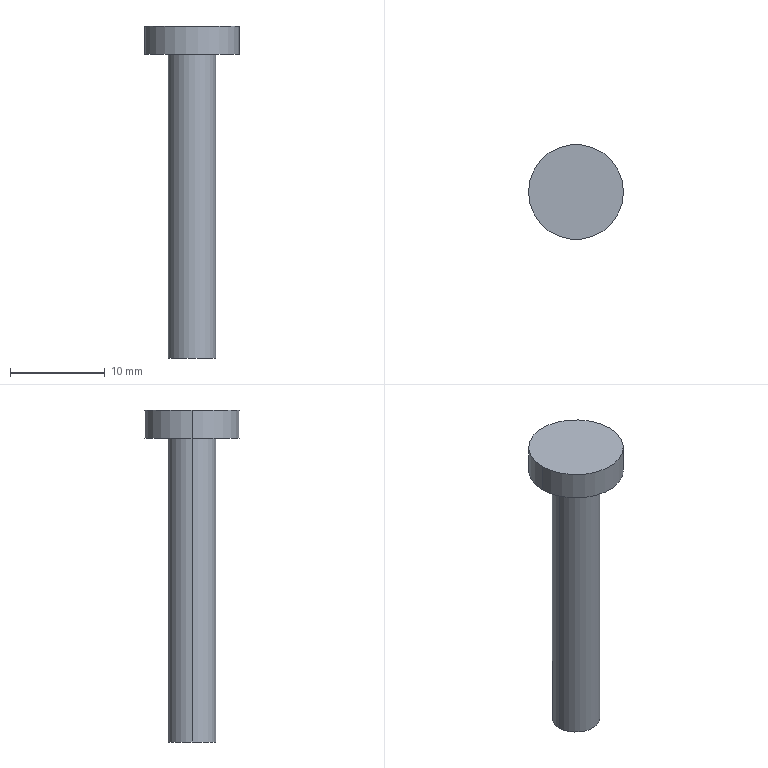Part | Creo | 1 solid | 7 faces | box 10 x 10 x 35 mm | volume 863.938 mm3 | cylinder 4 | plane 3 | commonest cylinder face diameters 5 x2 10 x2
STEP:
#1=CARTESIAN_POINT('',(-182.5,235.,-270.5));
#2=VERTEX_POINT('',#1);
#3=CARTESIAN_POINT('',(-187.5,235.,-270.5));
#4=VERTEX_POINT('',#3);
#5=CARTESIAN_POINT('',(-185.,235.,-270.5));
#6=DIRECTION('',(0.,0.,-1.));
#7=DIRECTION('',(1.,0.,0.));
#8=AXIS2_PLACEMENT_3D('',#5,#6,#7);
#9=CIRCLE('',#8,2.5);
#10=EDGE_CURVE('',#2,#4,#9,.T.);
#11=ORIENTED_EDGE('',*,*,#10,.T.);
#12=CARTESIAN_POINT('',(-187.5,235.,-238.5));
#13=VERTEX_POINT('',#12);
#14=CARTESIAN_POINT('',(-187.5,235.,-270.5));
#15=DIRECTION('',(0.,0.,1.));
#16=VECTOR('',#15,32.);
#17=LINE('',#14,#16);
#18=EDGE_CURVE('',#4,#13,#17,.T.);
#19=ORIENTED_EDGE('',*,*,#18,.T.);
#20=CARTESIAN_POINT('',(-182.5,235.,-238.5));
#21=VERTEX_POINT('',#20);
#22=CARTESIAN_POINT('',(-185.,235.,-238.5));
#23=DIRECTION('',(0.,0.,1.));
#24=DIRECTION('',(-1.,0.,0.));
#25=AXIS2_PLACEMENT_3D('',#22,#23,#24);
#26=CIRCLE('',#25,2.5);
#27=EDGE_CURVE('',#13,#21,#26,.T.);
#28=ORIENTED_EDGE('',*,*,#27,.T.);
#29=CARTESIAN_POINT('',(-182.5,235.,-270.5));
#30=DIRECTION('',(0.,0.,1.));
#31=VECTOR('',#30,32.);
#32=LINE('',#29,#31);
#33=EDGE_CURVE('',#2,#21,#32,.T.);
#34=ORIENTED_EDGE('',*,*,#33,.F.);
#35=EDGE_LOOP('',(#11,#19,#28,#34));
#36=FACE_OUTER_BOUND('',#35,.F.);
#37=CARTESIAN_POINT('',(-185.,235.,-520.5));
#38=DIRECTION('',(0.,0.,1.));
#39=DIRECTION('',(-1.,0.,0.));
#40=AXIS2_PLACEMENT_3D('',#37,#38,#39);
#41=CYLINDRICAL_SURFACE('',#40,2.5);
#42=ADVANCED_FACE('',(#36),#41,.T.);
#43=CARTESIAN_POINT('',(-185.,235.,-270.5));
#44=DIRECTION('',(0.,0.,-1.));
#45=DIRECTION('',(-1.,0.,0.));
#46=AXIS2_PLACEMENT_3D('',#43,#44,#45);
#47=CIRCLE('',#46,2.5);
#48=EDGE_CURVE('',#4,#2,#47,.T.);
#49=ORIENTED_EDGE('',*,*,#48,.F.);
#50=ORIENTED_EDGE('',*,*,#10,.F.);
#51=EDGE_LOOP('',(#49,#50));
#52=FACE_OUTER_BOUND('',#51,.F.);
#53=CARTESIAN_POINT('',(-476.957,8.569,-270.5));
#54=DIRECTION('',(0.,0.,-1.));
#55=DIRECTION('',(-1.,0.,0.));
#56=AXIS2_PLACEMENT_3D('',#53,#54,#55);
#57=PLANE('',#56);
#58=ADVANCED_FACE('',(#52),#57,.T.);
#59=ORIENTED_EDGE('',*,*,#48,.T.);
#60=ORIENTED_EDGE('',*,*,#33,.T.);
#61=CARTESIAN_POINT('',(-185.,235.,-238.5));
#62=DIRECTION('',(0.,0.,1.));
#63=DIRECTION('',(1.,0.,0.));
#64=AXIS2_PLACEMENT_3D('',#61,#62,#63);
#65=CIRCLE('',#64,2.5);
#66=EDGE_CURVE('',#21,#13,#65,.T.);
#67=ORIENTED_EDGE('',*,*,#66,.T.);
#68=ORIENTED_EDGE('',*,*,#18,.F.);
#69=EDGE_LOOP('',(#59,#60,#67,#68));
#70=FACE_OUTER_BOUND('',#69,.F.);
#71=CARTESIAN_POINT('',(-185.,235.,-520.5));
#72=DIRECTION('',(0.,0.,1.));
#73=DIRECTION('',(-1.,0.,0.));
#74=AXIS2_PLACEMENT_3D('',#71,#72,#73);
#75=CYLINDRICAL_SURFACE('',#74,2.5);
#76=ADVANCED_FACE('',(#70),#75,.T.);
#77=CARTESIAN_POINT('',(-180.,235.,-238.5));
#78=VERTEX_POINT('',#77);
#79=CARTESIAN_POINT('',(-190.,235.,-238.5));
#80=VERTEX_POINT('',#79);
#81=CARTESIAN_POINT('',(-185.,235.,-238.5));
#82=DIRECTION('',(0.,0.,-1.));
#83=DIRECTION('',(1.,0.,0.));
#84=AXIS2_PLACEMENT_3D('',#81,#82,#83);
#85=CIRCLE('',#84,5.);
#86=EDGE_CURVE('',#78,#80,#85,.T.);
#87=ORIENTED_EDGE('',*,*,#86,.F.);
#88=CARTESIAN_POINT('',(-185.,235.,-238.5));
#89=DIRECTION('',(0.,0.,-1.));
#90=DIRECTION('',(-1.,0.,0.));
#91=AXIS2_PLACEMENT_3D('',#88,#89,#90);
#92=CIRCLE('',#91,5.);
#93=EDGE_CURVE('',#80,#78,#92,.T.);
#94=ORIENTED_EDGE('',*,*,#93,.F.);
#95=EDGE_LOOP('',(#87,#94));
#96=FACE_OUTER_BOUND('',#95,.F.);
#97=ORIENTED_EDGE('',*,*,#66,.F.);
#98=ORIENTED_EDGE('',*,*,#27,.F.);
#99=EDGE_LOOP('',(#97,#98));
#100=FACE_BOUND('',#99,.F.);
#101=CARTESIAN_POINT('',(-185.,235.,-238.5));
#102=DIRECTION('',(0.,0.,1.));
#103=DIRECTION('',(-1.,0.,0.));
#104=AXIS2_PLACEMENT_3D('',#101,#102,#103);
#105=PLANE('',#104);
#106=ADVANCED_FACE('',(#96,#100),#105,.F.);
#107=CARTESIAN_POINT('',(-190.,235.,-235.5));
#108=VERTEX_POINT('',#107);
#109=CARTESIAN_POINT('',(-180.,235.,-235.5));
#110=VERTEX_POINT('',#109);
#111=CARTESIAN_POINT('',(-185.,235.,-235.5));
#112=DIRECTION('',(0.,0.,1.));
#113=DIRECTION('',(-1.,0.,0.));
#114=AXIS2_PLACEMENT_3D('',#111,#112,#113);
#115=CIRCLE('',#114,5.);
#116=EDGE_CURVE('',#108,#110,#115,.T.);
#117=ORIENTED_EDGE('',*,*,#116,.T.);
#118=CARTESIAN_POINT('',(-180.,235.,-238.5));
#119=DIRECTION('',(0.,0.,1.));
#120=VECTOR('',#119,3.);
#121=LINE('',#118,#120);
#122=EDGE_CURVE('',#78,#110,#121,.T.);
#123=ORIENTED_EDGE('',*,*,#122,.F.);
#124=ORIENTED_EDGE('',*,*,#86,.T.);
#125=CARTESIAN_POINT('',(-190.,235.,-238.5));
#126=DIRECTION('',(0.,0.,1.));
#127=VECTOR('',#126,3.);
#128=LINE('',#125,#127);
#129=EDGE_CURVE('',#80,#108,#128,.T.);
#130=ORIENTED_EDGE('',*,*,#129,.T.);
#131=EDGE_LOOP('',(#117,#123,#124,#130));
#132=FACE_OUTER_BOUND('',#131,.F.);
#133=CARTESIAN_POINT('',(-185.,235.,-225.087));
#134=DIRECTION('',(0.,0.,1.));
#135=DIRECTION('',(-1.,0.,0.));
#136=AXIS2_PLACEMENT_3D('',#133,#134,#135);
#137=CYLINDRICAL_SURFACE('',#136,5.);
#138=ADVANCED_FACE('',(#132),#137,.T.);
#139=ORIENTED_EDGE('',*,*,#116,.F.);
#140=CARTESIAN_POINT('',(-185.,235.,-235.5));
#141=DIRECTION('',(0.,0.,1.));
#142=DIRECTION('',(1.,0.,0.));
#143=AXIS2_PLACEMENT_3D('',#140,#141,#142);
#144=CIRCLE('',#143,5.);
#145=EDGE_CURVE('',#110,#108,#144,.T.);
#146=ORIENTED_EDGE('',*,*,#145,.F.);
#147=EDGE_LOOP('',(#139,#146));
#148=FACE_OUTER_BOUND('',#147,.F.);
#149=CARTESIAN_POINT('',(-181.,235.,-235.5));
#150=DIRECTION('',(0.,0.,-1.));
#151=DIRECTION('',(1.,0.,0.));
#152=AXIS2_PLACEMENT_3D('',#149,#150,#151);
#153=PLANE('',#152);
#154=ADVANCED_FACE('',(#148),#153,.F.);
#155=ORIENTED_EDGE('',*,*,#145,.T.);
#156=ORIENTED_EDGE('',*,*,#129,.F.);
#157=ORIENTED_EDGE('',*,*,#93,.T.);
#158=ORIENTED_EDGE('',*,*,#122,.T.);
#159=EDGE_LOOP('',(#155,#156,#157,#158));
#160=FACE_OUTER_BOUND('',#159,.F.);
#161=CARTESIAN_POINT('',(-185.,235.,-225.087));
#162=DIRECTION('',(0.,0.,1.));
#163=DIRECTION('',(-1.,0.,0.));
#164=AXIS2_PLACEMENT_3D('',#161,#162,#163);
#165=CYLINDRICAL_SURFACE('',#164,5.);
#166=ADVANCED_FACE('',(#160),#165,.T.);
#167=CLOSED_SHELL('',(#42,#58,#76,#106,#138,#154,#166));
#168=MANIFOLD_SOLID_BREP('',#167);
#169=(LENGTH_UNIT()NAMED_UNIT(*)SI_UNIT(.MILLI.,.METRE.));
#170=UNCERTAINTY_MEASURE_WITH_UNIT(LENGTH_MEASURE(0.003775),#169,'','');
#171=(NAMED_UNIT(*)PLANE_ANGLE_UNIT()SI_UNIT($,.RADIAN.));
#172=PLANE_ANGLE_MEASURE_WITH_UNIT(PLANE_ANGLE_MEASURE(0.01745),#171);
#173=(CONVERSION_BASED_UNIT('DEGREE',#172)NAMED_UNIT(*)PLANE_ANGLE_UNIT());
#174=(NAMED_UNIT(*)SI_UNIT($,.STERADIAN.)SOLID_ANGLE_UNIT());
#175=(GEOMETRIC_REPRESENTATION_CONTEXT(3)GLOBAL_UNCERTAINTY_ASSIGNED_CONTEXT((#170))GLOBAL_UNIT_ASSIGNED_CONTEXT((#169,#173,#174))REPRESENTATION_CONTEXT('',''));
#176=ADVANCED_BREP_SHAPE_REPRESENTATION('',(#168),#175);